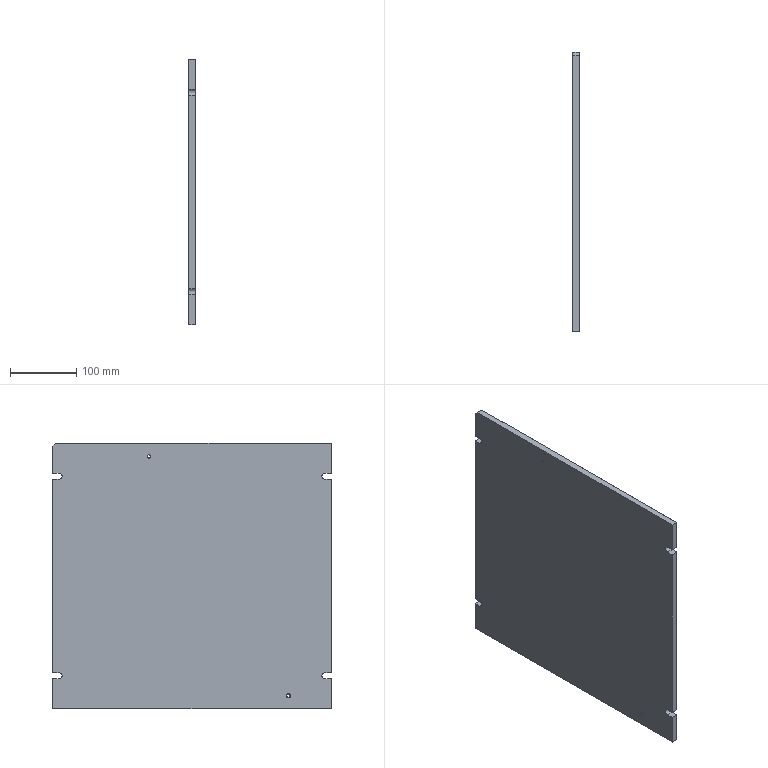Part | NX | 1 solid | 50 faces | box 10 x 420 x 400 mm | volume 1674456 mm3 | plane 38 | cylinder 8 | cone 4 | commonest cylinder face diameters 5 x4 9 x4
STEP:
#1=CARTESIAN_POINT('',(5.,-184.7,-204.5));
#2=VERTEX_POINT('',#1);
#3=CARTESIAN_POINT('',(5.,-184.7,-249.7));
#4=VERTEX_POINT('',#3);
#5=CARTESIAN_POINT('',(5.,-184.7,-227.25));
#6=DIRECTION('',(0.,0.,-1.));
#7=VECTOR('',#6,1000.);
#8=LINE('',#5,#7);
#9=EDGE_CURVE('',#2,#4,#8,.T.);
#10=ORIENTED_EDGE('',*,*,#9,.T.);
#11=CARTESIAN_POINT('',(5.,234.7,-249.7));
#12=VERTEX_POINT('',#11);
#13=CARTESIAN_POINT('',(5.,25.,-249.7));
#14=DIRECTION('',(0.,1.,0.));
#15=VECTOR('',#14,1000.);
#16=LINE('',#13,#15);
#17=EDGE_CURVE('',#4,#12,#16,.T.);
#18=ORIENTED_EDGE('',*,*,#17,.T.);
#19=CARTESIAN_POINT('',(5.,234.7,-204.5));
#20=VERTEX_POINT('',#19);
#21=CARTESIAN_POINT('',(5.,234.7,-227.25));
#22=DIRECTION('',(0.,0.,-1.));
#23=VECTOR('',#22,1000.);
#24=LINE('',#21,#23);
#25=EDGE_CURVE('',#20,#12,#24,.T.);
#26=ORIENTED_EDGE('',*,*,#25,.F.);
#27=CARTESIAN_POINT('',(5.,225.,-204.5));
#28=VERTEX_POINT('',#27);
#29=CARTESIAN_POINT('',(5.,0.,-204.5));
#30=DIRECTION('',(0.,1.,0.));
#31=VECTOR('',#30,1000.);
#32=LINE('',#29,#31);
#33=EDGE_CURVE('',#28,#20,#32,.T.);
#34=ORIENTED_EDGE('',*,*,#33,.F.);
#35=CARTESIAN_POINT('',(5.,225.,-195.5));
#36=VERTEX_POINT('',#35);
#37=CARTESIAN_POINT('',(5.,225.,-200.));
#38=DIRECTION('',(1.,0.,0.));
#39=DIRECTION('',(0.,0.,-1.));
#40=AXIS2_PLACEMENT_3D('',#37,#38,#39);
#41=CIRCLE('',#40,4.5);
#42=EDGE_CURVE('',#36,#28,#41,.T.);
#43=ORIENTED_EDGE('',*,*,#42,.F.);
#44=CARTESIAN_POINT('',(5.,234.7,-195.5));
#45=VERTEX_POINT('',#44);
#46=CARTESIAN_POINT('',(5.,0.,-195.5));
#47=DIRECTION('',(0.,-1.,0.));
#48=VECTOR('',#47,1000.);
#49=LINE('',#46,#48);
#50=EDGE_CURVE('',#45,#36,#49,.T.);
#51=ORIENTED_EDGE('',*,*,#50,.F.);
#52=CARTESIAN_POINT('',(5.,234.7,95.5));
#53=VERTEX_POINT('',#52);
#54=CARTESIAN_POINT('',(5.,234.7,-50.));
#55=DIRECTION('',(0.,0.,-1.));
#56=VECTOR('',#55,1000.);
#57=LINE('',#54,#56);
#58=EDGE_CURVE('',#53,#45,#57,.T.);
#59=ORIENTED_EDGE('',*,*,#58,.F.);
#60=CARTESIAN_POINT('',(5.,225.,95.5));
#61=VERTEX_POINT('',#60);
#62=CARTESIAN_POINT('',(5.,0.,95.5));
#63=DIRECTION('',(0.,1.,0.));
#64=VECTOR('',#63,1000.);
#65=LINE('',#62,#64);
#66=EDGE_CURVE('',#61,#53,#65,.T.);
#67=ORIENTED_EDGE('',*,*,#66,.F.);
#68=CARTESIAN_POINT('',(5.,225.,104.5));
#69=VERTEX_POINT('',#68);
#70=CARTESIAN_POINT('',(5.,225.,100.));
#71=DIRECTION('',(1.,0.,0.));
#72=DIRECTION('',(0.,0.,-1.));
#73=AXIS2_PLACEMENT_3D('',#70,#71,#72);
#74=CIRCLE('',#73,4.5);
#75=EDGE_CURVE('',#69,#61,#74,.T.);
#76=ORIENTED_EDGE('',*,*,#75,.F.);
#77=CARTESIAN_POINT('',(5.,234.7,104.5));
#78=VERTEX_POINT('',#77);
#79=CARTESIAN_POINT('',(5.,0.,104.5));
#80=DIRECTION('',(0.,-1.,0.));
#81=VECTOR('',#80,1000.);
#82=LINE('',#79,#81);
#83=EDGE_CURVE('',#78,#69,#82,.T.);
#84=ORIENTED_EDGE('',*,*,#83,.F.);
#85=CARTESIAN_POINT('',(5.,234.7,145.3));
#86=VERTEX_POINT('',#85);
#87=CARTESIAN_POINT('',(5.,234.7,124.75));
#88=DIRECTION('',(0.,0.,-1.));
#89=VECTOR('',#88,1000.);
#90=LINE('',#87,#89);
#91=EDGE_CURVE('',#86,#78,#90,.T.);
#92=ORIENTED_EDGE('',*,*,#91,.F.);
#93=CARTESIAN_POINT('',(5.,230.3,149.7));
#94=VERTEX_POINT('',#93);
#95=CARTESIAN_POINT('',(5.,380.,0.));
#96=DIRECTION('',(0.,0.7071,-0.7071));
#97=VECTOR('',#96,1000.);
#98=LINE('',#95,#97);
#99=EDGE_CURVE('',#94,#86,#98,.T.);
#100=ORIENTED_EDGE('',*,*,#99,.F.);
#101=CARTESIAN_POINT('',(5.,-184.7,149.7));
#102=VERTEX_POINT('',#101);
#103=CARTESIAN_POINT('',(5.,22.5,149.7));
#104=DIRECTION('',(0.,1.,0.));
#105=VECTOR('',#104,1000.);
#106=LINE('',#103,#105);
#107=EDGE_CURVE('',#102,#94,#106,.T.);
#108=ORIENTED_EDGE('',*,*,#107,.F.);
#109=CARTESIAN_POINT('',(5.,-184.7,104.5));
#110=VERTEX_POINT('',#109);
#111=CARTESIAN_POINT('',(5.,-184.7,127.25));
#112=DIRECTION('',(0.,0.,-1.));
#113=VECTOR('',#112,1000.);
#114=LINE('',#111,#113);
#115=EDGE_CURVE('',#102,#110,#114,.T.);
#116=ORIENTED_EDGE('',*,*,#115,.T.);
#117=CARTESIAN_POINT('',(5.,-175.,104.5));
#118=VERTEX_POINT('',#117);
#119=CARTESIAN_POINT('',(5.,0.,104.5));
#120=DIRECTION('',(0.,-1.,0.));
#121=VECTOR('',#120,1000.);
#122=LINE('',#119,#121);
#123=EDGE_CURVE('',#118,#110,#122,.T.);
#124=ORIENTED_EDGE('',*,*,#123,.F.);
#125=CARTESIAN_POINT('',(5.,-175.,95.5));
#126=VERTEX_POINT('',#125);
#127=CARTESIAN_POINT('',(5.,-175.,100.));
#128=DIRECTION('',(1.,0.,0.));
#129=DIRECTION('',(0.,0.,-1.));
#130=AXIS2_PLACEMENT_3D('',#127,#128,#129);
#131=CIRCLE('',#130,4.5);
#132=EDGE_CURVE('',#126,#118,#131,.T.);
#133=ORIENTED_EDGE('',*,*,#132,.F.);
#134=CARTESIAN_POINT('',(5.,-184.7,95.5));
#135=VERTEX_POINT('',#134);
#136=CARTESIAN_POINT('',(5.,0.,95.5));
#137=DIRECTION('',(0.,1.,0.));
#138=VECTOR('',#137,1000.);
#139=LINE('',#136,#138);
#140=EDGE_CURVE('',#135,#126,#139,.T.);
#141=ORIENTED_EDGE('',*,*,#140,.F.);
#142=CARTESIAN_POINT('',(5.,-184.7,-195.5));
#143=VERTEX_POINT('',#142);
#144=CARTESIAN_POINT('',(5.,-184.7,-50.));
#145=DIRECTION('',(0.,0.,-1.));
#146=VECTOR('',#145,1000.);
#147=LINE('',#144,#146);
#148=EDGE_CURVE('',#135,#143,#147,.T.);
#149=ORIENTED_EDGE('',*,*,#148,.T.);
#150=CARTESIAN_POINT('',(5.,-175.,-195.5));
#151=VERTEX_POINT('',#150);
#152=CARTESIAN_POINT('',(5.,0.,-195.5));
#153=DIRECTION('',(0.,-1.,0.));
#154=VECTOR('',#153,1000.);
#155=LINE('',#152,#154);
#156=EDGE_CURVE('',#151,#143,#155,.T.);
#157=ORIENTED_EDGE('',*,*,#156,.F.);
#158=CARTESIAN_POINT('',(5.,-175.,-204.5));
#159=VERTEX_POINT('',#158);
#160=CARTESIAN_POINT('',(5.,-175.,-200.));
#161=DIRECTION('',(1.,0.,0.));
#162=DIRECTION('',(0.,0.,-1.));
#163=AXIS2_PLACEMENT_3D('',#160,#161,#162);
#164=CIRCLE('',#163,4.5);
#165=EDGE_CURVE('',#159,#151,#164,.T.);
#166=ORIENTED_EDGE('',*,*,#165,.F.);
#167=CARTESIAN_POINT('',(5.,0.,-204.5));
#168=DIRECTION('',(0.,1.,0.));
#169=VECTOR('',#168,1000.);
#170=LINE('',#167,#169);
#171=EDGE_CURVE('',#2,#159,#170,.T.);
#172=ORIENTED_EDGE('',*,*,#171,.F.);
#173=EDGE_LOOP('',(#10,#18,#26,#34,#43,#51,#59,#67,#76,#84,#92,#100,#108,#116,#124,#133,#141,#149,#157,#166,#172));
#174=FACE_BOUND('',#173,.T.);
#175=CARTESIAN_POINT('',(5.,93.45,130.));
#176=VERTEX_POINT('',#175);
#177=CARTESIAN_POINT('',(5.,86.55,130.));
#178=VERTEX_POINT('',#177);
#179=CARTESIAN_POINT('',(5.,90.,130.));
#180=DIRECTION('',(1.,0.,0.));
#181=DIRECTION('',(0.,-1.,0.));
#182=AXIS2_PLACEMENT_3D('',#179,#180,#181);
#183=CIRCLE('',#182,3.45);
#184=EDGE_CURVE('',#176,#178,#183,.T.);
#185=ORIENTED_EDGE('',*,*,#184,.F.);
#186=CARTESIAN_POINT('',(5.,90.,130.));
#187=DIRECTION('',(1.,0.,0.));
#188=DIRECTION('',(0.,-1.,0.));
#189=AXIS2_PLACEMENT_3D('',#186,#187,#188);
#190=CIRCLE('',#189,3.45);
#191=EDGE_CURVE('',#178,#176,#190,.T.);
#192=ORIENTED_EDGE('',*,*,#191,.F.);
#193=EDGE_LOOP('',(#185,#192));
#194=FACE_BOUND('',#193,.T.);
#195=CARTESIAN_POINT('',(5.,-122.5,-230.));
#196=VERTEX_POINT('',#195);
#197=CARTESIAN_POINT('',(5.,-117.5,-230.));
#198=VERTEX_POINT('',#197);
#199=CARTESIAN_POINT('',(5.,-120.,-230.));
#200=DIRECTION('',(-1.,0.,0.));
#201=DIRECTION('',(0.,1.,0.));
#202=AXIS2_PLACEMENT_3D('',#199,#200,#201);
#203=CIRCLE('',#202,2.5);
#204=EDGE_CURVE('',#196,#198,#203,.T.);
#205=ORIENTED_EDGE('',*,*,#204,.T.);
#206=CARTESIAN_POINT('',(5.,-120.,-230.));
#207=DIRECTION('',(-1.,0.,0.));
#208=DIRECTION('',(0.,1.,0.));
#209=AXIS2_PLACEMENT_3D('',#206,#207,#208);
#210=CIRCLE('',#209,2.5);
#211=EDGE_CURVE('',#198,#196,#210,.T.);
#212=ORIENTED_EDGE('',*,*,#211,.T.);
#213=EDGE_LOOP('',(#205,#212));
#214=FACE_BOUND('',#213,.T.);
#215=CARTESIAN_POINT('',(5.,0.,0.));
#216=DIRECTION('',(1.,0.,0.));
#217=DIRECTION('',(0.,1.,0.));
#218=AXIS2_PLACEMENT_3D('',#215,#216,#217);
#219=PLANE('',#218);
#220=ADVANCED_FACE('',(#174,#194,#214),#219,.T.);
#221=CARTESIAN_POINT('',(-4.7,-184.7,150.));
#222=VERTEX_POINT('',#221);
#223=CARTESIAN_POINT('',(4.7,-184.7,150.));
#224=VERTEX_POINT('',#223);
#225=CARTESIAN_POINT('',(0.,-184.7,150.));
#226=DIRECTION('',(1.,0.,0.));
#227=VECTOR('',#226,1000.);
#228=LINE('',#225,#227);
#229=EDGE_CURVE('',#222,#224,#228,.T.);
#230=ORIENTED_EDGE('',*,*,#229,.T.);
#231=CARTESIAN_POINT('',(4.7,230.,150.));
#232=VERTEX_POINT('',#231);
#233=CARTESIAN_POINT('',(4.7,22.5,150.));
#234=DIRECTION('',(0.,1.,0.));
#235=VECTOR('',#234,1000.);
#236=LINE('',#233,#235);
#237=EDGE_CURVE('',#224,#232,#236,.T.);
#238=ORIENTED_EDGE('',*,*,#237,.T.);
#239=CARTESIAN_POINT('',(-4.7,230.,150.));
#240=VERTEX_POINT('',#239);
#241=CARTESIAN_POINT('',(5.,230.,150.));
#242=DIRECTION('',(-1.,0.,0.));
#243=VECTOR('',#242,1000.);
#244=LINE('',#241,#243);
#245=EDGE_CURVE('',#232,#240,#244,.T.);
#246=ORIENTED_EDGE('',*,*,#245,.T.);
#247=CARTESIAN_POINT('',(-4.7,22.5,150.));
#248=DIRECTION('',(0.,1.,0.));
#249=VECTOR('',#248,1000.);
#250=LINE('',#247,#249);
#251=EDGE_CURVE('',#222,#240,#250,.T.);
#252=ORIENTED_EDGE('',*,*,#251,.F.);
#253=EDGE_LOOP('',(#230,#238,#246,#252));
#254=FACE_BOUND('',#253,.T.);
#255=CARTESIAN_POINT('',(-5.,235.,150.));
#256=DIRECTION('',(0.,0.,1.));
#257=DIRECTION('',(1.,0.,0.));
#258=AXIS2_PLACEMENT_3D('',#255,#256,#257);
#259=PLANE('',#258);
#260=ADVANCED_FACE('',(#254),#259,.T.);
#261=ORIENTED_EDGE('',*,*,#245,.F.);
#262=CARTESIAN_POINT('',(154.7,380.,0.));
#263=DIRECTION('',(0.5774,0.5774,-0.5774));
#264=VECTOR('',#263,1000.);
#265=LINE('',#262,#264);
#266=EDGE_CURVE('',#232,#94,#265,.T.);
#267=ORIENTED_EDGE('',*,*,#266,.T.);
#268=ORIENTED_EDGE('',*,*,#99,.T.);
#269=CARTESIAN_POINT('',(4.7,235.,145.));
#270=VERTEX_POINT('',#269);
#271=CARTESIAN_POINT('',(239.7,0.,380.));
#272=DIRECTION('',(-0.5774,0.5774,-0.5774));
#273=VECTOR('',#272,1000.);
#274=LINE('',#271,#273);
#275=EDGE_CURVE('',#86,#270,#274,.T.);
#276=ORIENTED_EDGE('',*,*,#275,.T.);
#277=CARTESIAN_POINT('',(-4.7,235.,145.));
#278=VERTEX_POINT('',#277);
#279=CARTESIAN_POINT('',(5.,235.,145.));
#280=DIRECTION('',(-1.,0.,0.));
#281=VECTOR('',#280,1000.);
#282=LINE('',#279,#281);
#283=EDGE_CURVE('',#270,#278,#282,.T.);
#284=ORIENTED_EDGE('',*,*,#283,.T.);
#285=CARTESIAN_POINT('',(-5.,234.7,145.3));
#286=VERTEX_POINT('',#285);
#287=CARTESIAN_POINT('',(140.3,380.,0.));
#288=DIRECTION('',(0.5774,0.5774,-0.5774));
#289=VECTOR('',#288,1000.);
#290=LINE('',#287,#289);
#291=EDGE_CURVE('',#286,#278,#290,.T.);
#292=ORIENTED_EDGE('',*,*,#291,.F.);
#293=CARTESIAN_POINT('',(-5.,230.3,149.7));
#294=VERTEX_POINT('',#293);
#295=CARTESIAN_POINT('',(-5.,380.,0.));
#296=DIRECTION('',(0.,0.7071,-0.7071));
#297=VECTOR('',#296,1000.);
#298=LINE('',#295,#297);
#299=EDGE_CURVE('',#294,#286,#298,.T.);
#300=ORIENTED_EDGE('',*,*,#299,.F.);
#301=CARTESIAN_POINT('',(-154.7,380.,0.));
#302=DIRECTION('',(-0.5774,0.5774,-0.5774));
#303=VECTOR('',#302,1000.);
#304=LINE('',#301,#303);
#305=EDGE_CURVE('',#240,#294,#304,.T.);
#306=ORIENTED_EDGE('',*,*,#305,.F.);
#307=EDGE_LOOP('',(#261,#267,#268,#276,#284,#292,#300,#306));
#308=FACE_BOUND('',#307,.T.);
#309=CARTESIAN_POINT('',(-5.,230.,150.));
#310=DIRECTION('',(0.,0.7071,0.7071));
#311=DIRECTION('',(1.,0.,0.));
#312=AXIS2_PLACEMENT_3D('',#309,#310,#311);
#313=PLANE('',#312);
#314=ADVANCED_FACE('',(#308),#313,.T.);
#315=CARTESIAN_POINT('',(4.7,235.,-249.7));
#316=VERTEX_POINT('',#315);
#317=CARTESIAN_POINT('',(-4.7,235.,-249.7));
#318=VERTEX_POINT('',#317);
#319=CARTESIAN_POINT('',(0.,235.,-249.7));
#320=DIRECTION('',(-1.,0.,0.));
#321=VECTOR('',#320,1000.);
#322=LINE('',#319,#321);
#323=EDGE_CURVE('',#316,#318,#322,.T.);
#324=ORIENTED_EDGE('',*,*,#323,.T.);
#325=CARTESIAN_POINT('',(-4.7,235.,-204.5));
#326=VERTEX_POINT('',#325);
#327=CARTESIAN_POINT('',(-4.7,235.,-227.25));
#328=DIRECTION('',(0.,0.,-1.));
#329=VECTOR('',#328,1000.);
#330=LINE('',#327,#329);
#331=EDGE_CURVE('',#326,#318,#330,.T.);
#332=ORIENTED_EDGE('',*,*,#331,.F.);
#333=CARTESIAN_POINT('',(4.7,235.,-204.5));
#334=VERTEX_POINT('',#333);
#335=CARTESIAN_POINT('',(-6.,235.,-204.5));
#336=DIRECTION('',(1.,0.,0.));
#337=VECTOR('',#336,1000.);
#338=LINE('',#335,#337);
#339=EDGE_CURVE('',#326,#334,#338,.T.);
#340=ORIENTED_EDGE('',*,*,#339,.T.);
#341=CARTESIAN_POINT('',(4.7,235.,-227.25));
#342=DIRECTION('',(0.,0.,-1.));
#343=VECTOR('',#342,1000.);
#344=LINE('',#341,#343);
#345=EDGE_CURVE('',#334,#316,#344,.T.);
#346=ORIENTED_EDGE('',*,*,#345,.T.);
#347=EDGE_LOOP('',(#324,#332,#340,#346));
#348=FACE_BOUND('',#347,.T.);
#349=CARTESIAN_POINT('',(-5.,235.,-150.));
#350=DIRECTION('',(0.,1.,0.));
#351=DIRECTION('',(1.,0.,0.));
#352=AXIS2_PLACEMENT_3D('',#349,#350,#351);
#353=PLANE('',#352);
#354=ADVANCED_FACE('',(#348),#353,.T.);
#355=CARTESIAN_POINT('',(-4.7,235.,104.5));
#356=VERTEX_POINT('',#355);
#357=CARTESIAN_POINT('',(4.7,235.,104.5));
#358=VERTEX_POINT('',#357);
#359=CARTESIAN_POINT('',(-6.,235.,104.5));
#360=DIRECTION('',(1.,0.,0.));
#361=VECTOR('',#360,1000.);
#362=LINE('',#359,#361);
#363=EDGE_CURVE('',#356,#358,#362,.T.);
#364=ORIENTED_EDGE('',*,*,#363,.F.);
#365=CARTESIAN_POINT('',(-4.7,235.,124.75));
#366=DIRECTION('',(0.,0.,-1.));
#367=VECTOR('',#366,1000.);
#368=LINE('',#365,#367);
#369=EDGE_CURVE('',#278,#356,#368,.T.);
#370=ORIENTED_EDGE('',*,*,#369,.F.);
#371=ORIENTED_EDGE('',*,*,#283,.F.);
#372=CARTESIAN_POINT('',(4.7,235.,124.75));
#373=DIRECTION('',(0.,0.,-1.));
#374=VECTOR('',#373,1000.);
#375=LINE('',#372,#374);
#376=EDGE_CURVE('',#270,#358,#375,.T.);
#377=ORIENTED_EDGE('',*,*,#376,.T.);
#378=EDGE_LOOP('',(#364,#370,#371,#377));
#379=FACE_BOUND('',#378,.T.);
#380=CARTESIAN_POINT('',(-5.,235.,-150.));
#381=DIRECTION('',(0.,1.,0.));
#382=DIRECTION('',(1.,0.,0.));
#383=AXIS2_PLACEMENT_3D('',#380,#381,#382);
#384=PLANE('',#383);
#385=ADVANCED_FACE('',(#379),#384,.T.);
#386=CARTESIAN_POINT('',(4.7,-184.7,-250.));
#387=VERTEX_POINT('',#386);
#388=CARTESIAN_POINT('',(-4.7,-184.7,-250.));
#389=VERTEX_POINT('',#388);
#390=CARTESIAN_POINT('',(0.,-184.7,-250.));
#391=DIRECTION('',(-1.,0.,0.));
#392=VECTOR('',#391,1000.);
#393=LINE('',#390,#392);
#394=EDGE_CURVE('',#387,#389,#393,.T.);
#395=ORIENTED_EDGE('',*,*,#394,.T.);
#396=CARTESIAN_POINT('',(-4.7,234.7,-250.));
#397=VERTEX_POINT('',#396);
#398=CARTESIAN_POINT('',(-4.7,25.,-250.));
#399=DIRECTION('',(0.,1.,0.));
#400=VECTOR('',#399,1000.);
#401=LINE('',#398,#400);
#402=EDGE_CURVE('',#389,#397,#401,.T.);
#403=ORIENTED_EDGE('',*,*,#402,.T.);
#404=CARTESIAN_POINT('',(4.7,234.7,-250.));
#405=VERTEX_POINT('',#404);
#406=CARTESIAN_POINT('',(0.,234.7,-250.));
#407=DIRECTION('',(-1.,0.,0.));
#408=VECTOR('',#407,1000.);
#409=LINE('',#406,#408);
#410=EDGE_CURVE('',#405,#397,#409,.T.);
#411=ORIENTED_EDGE('',*,*,#410,.F.);
#412=CARTESIAN_POINT('',(4.7,25.,-250.));
#413=DIRECTION('',(0.,1.,0.));
#414=VECTOR('',#413,1000.);
#415=LINE('',#412,#414);
#416=EDGE_CURVE('',#387,#405,#415,.T.);
#417=ORIENTED_EDGE('',*,*,#416,.F.);
#418=EDGE_LOOP('',(#395,#403,#411,#417));
#419=FACE_BOUND('',#418,.T.);
#420=CARTESIAN_POINT('',(-5.,-235.,-250.));
#421=DIRECTION('',(0.,0.,-1.));
#422=DIRECTION('',(0.,-1.,0.));
#423=AXIS2_PLACEMENT_3D('',#420,#421,#422);
#424=PLANE('',#423);
#425=ADVANCED_FACE('',(#419),#424,.T.);
#426=CARTESIAN_POINT('',(-5.,225.,-204.5));
#427=VERTEX_POINT('',#426);
#428=CARTESIAN_POINT('',(-5.,234.7,-204.5));
#429=VERTEX_POINT('',#428);
#430=CARTESIAN_POINT('',(-5.,0.,-204.5));
#431=DIRECTION('',(0.,1.,0.));
#432=VECTOR('',#431,1000.);
#433=LINE('',#430,#432);
#434=EDGE_CURVE('',#427,#429,#433,.T.);
#435=ORIENTED_EDGE('',*,*,#434,.F.);
#436=CARTESIAN_POINT('',(-6.,225.,-204.5));
#437=DIRECTION('',(1.,0.,0.));
#438=VECTOR('',#437,1000.);
#439=LINE('',#436,#438);
#440=EDGE_CURVE('',#427,#28,#439,.T.);
#441=ORIENTED_EDGE('',*,*,#440,.T.);
#442=ORIENTED_EDGE('',*,*,#33,.T.);
#443=CARTESIAN_POINT('',(239.7,0.,-204.5));
#444=DIRECTION('',(0.7071,-0.7071,0.));
#445=VECTOR('',#444,1000.);
#446=LINE('',#443,#445);
#447=EDGE_CURVE('',#334,#20,#446,.T.);
#448=ORIENTED_EDGE('',*,*,#447,.F.);
#449=ORIENTED_EDGE('',*,*,#339,.F.);
#450=CARTESIAN_POINT('',(-239.7,0.,-204.5));
#451=DIRECTION('',(-0.7071,-0.7071,0.));
#452=VECTOR('',#451,1000.);
#453=LINE('',#450,#452);
#454=EDGE_CURVE('',#326,#429,#453,.T.);
#455=ORIENTED_EDGE('',*,*,#454,.T.);
#456=EDGE_LOOP('',(#435,#441,#442,#448,#449,#455));
#457=FACE_BOUND('',#456,.T.);
#458=CARTESIAN_POINT('',(-6.,235.,-204.5));
#459=DIRECTION('',(0.,0.,-1.));
#460=DIRECTION('',(0.,-1.,0.));
#461=AXIS2_PLACEMENT_3D('',#458,#459,#460);
#462=PLANE('',#461);
#463=ADVANCED_FACE('',(#457),#462,.F.);
#464=CARTESIAN_POINT('',(-4.7,-185.,-204.5));
#465=VERTEX_POINT('',#464);
#466=CARTESIAN_POINT('',(-4.7,-185.,-249.7));
#467=VERTEX_POINT('',#466);
#468=CARTESIAN_POINT('',(-4.7,-185.,-227.25));
#469=DIRECTION('',(0.,0.,-1.));
#470=VECTOR('',#469,1000.);
#471=LINE('',#468,#470);
#472=EDGE_CURVE('',#465,#467,#471,.T.);
#473=ORIENTED_EDGE('',*,*,#472,.T.);
#474=CARTESIAN_POINT('',(4.7,-185.,-249.7));
#475=VERTEX_POINT('',#474);
#476=CARTESIAN_POINT('',(0.,-185.,-249.7));
#477=DIRECTION('',(-1.,0.,0.));
#478=VECTOR('',#477,1000.);
#479=LINE('',#476,#478);
#480=EDGE_CURVE('',#475,#467,#479,.T.);
#481=ORIENTED_EDGE('',*,*,#480,.F.);
#482=CARTESIAN_POINT('',(4.7,-185.,-204.5));
#483=VERTEX_POINT('',#482);
#484=CARTESIAN_POINT('',(4.7,-185.,-227.25));
#485=DIRECTION('',(0.,0.,-1.));
#486=VECTOR('',#485,1000.);
#487=LINE('',#484,#486);
#488=EDGE_CURVE('',#483,#475,#487,.T.);
#489=ORIENTED_EDGE('',*,*,#488,.F.);
#490=CARTESIAN_POINT('',(0.,-185.,-204.5));
#491=DIRECTION('',(-1.,0.,0.));
#492=VECTOR('',#491,1000.);
#493=LINE('',#490,#492);
#494=EDGE_CURVE('',#483,#465,#493,.T.);
#495=ORIENTED_EDGE('',*,*,#494,.T.);
#496=EDGE_LOOP('',(#473,#481,#489,#495));
#497=FACE_BOUND('',#496,.T.);
#498=CARTESIAN_POINT('',(-5.,-185.,150.));
#499=DIRECTION('',(0.,-1.,0.));
#500=DIRECTION('',(0.,0.,-1.));
#501=AXIS2_PLACEMENT_3D('',#498,#499,#500);
#502=PLANE('',#501);
#503=ADVANCED_FACE('',(#497),#502,.T.);
#504=CARTESIAN_POINT('',(4.452,92.5,130.));
#505=VERTEX_POINT('',#504);
#506=CARTESIAN_POINT('',(4.452,87.5,130.));
#507=VERTEX_POINT('',#506);
#508=CARTESIAN_POINT('',(4.452,90.,130.));
#509=DIRECTION('',(1.,0.,0.));
#510=DIRECTION('',(0.,-1.,0.));
#511=AXIS2_PLACEMENT_3D('',#508,#509,#510);
#512=CIRCLE('',#511,2.5);
#513=EDGE_CURVE('',#505,#507,#512,.T.);
#514=ORIENTED_EDGE('',*,*,#513,.T.);
#515=CARTESIAN_POINT('',(-5.,87.5,130.));
#516=VERTEX_POINT('',#515);
#517=CARTESIAN_POINT('',(5.,87.5,130.));
#518=DIRECTION('',(1.,0.,0.));
#519=VECTOR('',#518,1000.);
#520=LINE('',#517,#519);
#521=EDGE_CURVE('',#507,#516,#520,.F.);
#522=ORIENTED_EDGE('',*,*,#521,.T.);
#523=CARTESIAN_POINT('',(-5.,92.5,130.));
#524=VERTEX_POINT('',#523);
#525=CARTESIAN_POINT('',(-5.,90.,130.));
#526=DIRECTION('',(1.,0.,0.));
#527=DIRECTION('',(0.,-1.,0.));
#528=AXIS2_PLACEMENT_3D('',#525,#526,#527);
#529=CIRCLE('',#528,2.5);
#530=EDGE_CURVE('',#524,#516,#529,.T.);
#531=ORIENTED_EDGE('',*,*,#530,.F.);
#532=CARTESIAN_POINT('',(5.,92.5,130.));
#533=DIRECTION('',(1.,0.,0.));
#534=VECTOR('',#533,1000.);
#535=LINE('',#532,#534);
#536=EDGE_CURVE('',#505,#524,#535,.F.);
#537=ORIENTED_EDGE('',*,*,#536,.F.);
#538=EDGE_LOOP('',(#514,#522,#531,#537));
#539=FACE_BOUND('',#538,.T.);
#540=CARTESIAN_POINT('',(5.,90.,130.));
#541=DIRECTION('',(1.,0.,0.));
#542=DIRECTION('',(0.,-1.,0.));
#543=AXIS2_PLACEMENT_3D('',#540,#541,#542);
#544=CYLINDRICAL_SURFACE('',#543,2.5);
#545=ADVANCED_FACE('',(#539),#544,.F.);
#546=CARTESIAN_POINT('',(-5.,-184.7,-204.5));
#547=VERTEX_POINT('',#546);
#548=CARTESIAN_POINT('',(-5.,-184.7,-249.7));
#549=VERTEX_POINT('',#548);
#550=CARTESIAN_POINT('',(-5.,-184.7,-227.25));
#551=DIRECTION('',(0.,0.,-1.));
#552=VECTOR('',#551,1000.);
#553=LINE('',#550,#552);
#554=EDGE_CURVE('',#547,#549,#553,.T.);
#555=ORIENTED_EDGE('',*,*,#554,.F.);
#556=CARTESIAN_POINT('',(-5.,-175.,-204.5));
#557=VERTEX_POINT('',#556);
#558=CARTESIAN_POINT('',(-5.,0.,-204.5));
#559=DIRECTION('',(0.,1.,0.));
#560=VECTOR('',#559,1000.);
#561=LINE('',#558,#560);
#562=EDGE_CURVE('',#547,#557,#561,.T.);
#563=ORIENTED_EDGE('',*,*,#562,.T.);
#564=CARTESIAN_POINT('',(-5.,-175.,-195.5));
#565=VERTEX_POINT('',#564);
#566=CARTESIAN_POINT('',(-5.,-175.,-200.));
#567=DIRECTION('',(1.,0.,0.));
#568=DIRECTION('',(0.,0.,-1.));
#569=AXIS2_PLACEMENT_3D('',#566,#567,#568);
#570=CIRCLE('',#569,4.5);
#571=EDGE_CURVE('',#557,#565,#570,.T.);
#572=ORIENTED_EDGE('',*,*,#571,.T.);
#573=CARTESIAN_POINT('',(-5.,-184.7,-195.5));
#574=VERTEX_POINT('',#573);
#575=CARTESIAN_POINT('',(-5.,0.,-195.5));
#576=DIRECTION('',(0.,-1.,0.));
#577=VECTOR('',#576,1000.);
#578=LINE('',#575,#577);
#579=EDGE_CURVE('',#565,#574,#578,.T.);
#580=ORIENTED_EDGE('',*,*,#579,.T.);
#581=CARTESIAN_POINT('',(-5.,-184.7,95.5));
#582=VERTEX_POINT('',#581);
#583=CARTESIAN_POINT('',(-5.,-184.7,-50.));
#584=DIRECTION('',(0.,0.,-1.));
#585=VECTOR('',#584,1000.);
#586=LINE('',#583,#585);
#587=EDGE_CURVE('',#582,#574,#586,.T.);
#588=ORIENTED_EDGE('',*,*,#587,.F.);
#589=CARTESIAN_POINT('',(-5.,-175.,95.5));
#590=VERTEX_POINT('',#589);
#591=CARTESIAN_POINT('',(-5.,0.,95.5));
#592=DIRECTION('',(0.,1.,0.));
#593=VECTOR('',#592,1000.);
#594=LINE('',#591,#593);
#595=EDGE_CURVE('',#582,#590,#594,.T.);
#596=ORIENTED_EDGE('',*,*,#595,.T.);
#597=CARTESIAN_POINT('',(-5.,-175.,104.5));
#598=VERTEX_POINT('',#597);
#599=CARTESIAN_POINT('',(-5.,-175.,100.));
#600=DIRECTION('',(1.,0.,0.));
#601=DIRECTION('',(0.,0.,-1.));
#602=AXIS2_PLACEMENT_3D('',#599,#600,#601);
#603=CIRCLE('',#602,4.5);
#604=EDGE_CURVE('',#590,#598,#603,.T.);
#605=ORIENTED_EDGE('',*,*,#604,.T.);
#606=CARTESIAN_POINT('',(-5.,-184.7,104.5));
#607=VERTEX_POINT('',#606);
#608=CARTESIAN_POINT('',(-5.,0.,104.5));
#609=DIRECTION('',(0.,-1.,0.));
#610=VECTOR('',#609,1000.);
#611=LINE('',#608,#610);
#612=EDGE_CURVE('',#598,#607,#611,.T.);
#613=ORIENTED_EDGE('',*,*,#612,.T.);
#614=CARTESIAN_POINT('',(-5.,-184.7,149.7));
#615=VERTEX_POINT('',#614);
#616=CARTESIAN_POINT('',(-5.,-184.7,127.25));
#617=DIRECTION('',(0.,0.,-1.));
#618=VECTOR('',#617,1000.);
#619=LINE('',#616,#618);
#620=EDGE_CURVE('',#615,#607,#619,.T.);
#621=ORIENTED_EDGE('',*,*,#620,.F.);
#622=CARTESIAN_POINT('',(-5.,22.5,149.7));
#623=DIRECTION('',(0.,1.,0.));
#624=VECTOR('',#623,1000.);
#625=LINE('',#622,#624);
#626=EDGE_CURVE('',#615,#294,#625,.T.);
#627=ORIENTED_EDGE('',*,*,#626,.T.);
#628=ORIENTED_EDGE('',*,*,#299,.T.);
#629=CARTESIAN_POINT('',(-5.,234.7,104.5));
#630=VERTEX_POINT('',#629);
#631=CARTESIAN_POINT('',(-5.,234.7,124.75));
#632=DIRECTION('',(0.,0.,-1.));
#633=VECTOR('',#632,1000.);
#634=LINE('',#631,#633);
#635=EDGE_CURVE('',#286,#630,#634,.T.);
#636=ORIENTED_EDGE('',*,*,#635,.T.);
#637=CARTESIAN_POINT('',(-5.,225.,104.5));
#638=VERTEX_POINT('',#637);
#639=CARTESIAN_POINT('',(-5.,0.,104.5));
#640=DIRECTION('',(0.,-1.,0.));
#641=VECTOR('',#640,1000.);
#642=LINE('',#639,#641);
#643=EDGE_CURVE('',#630,#638,#642,.T.);
#644=ORIENTED_EDGE('',*,*,#643,.T.);
#645=CARTESIAN_POINT('',(-5.,225.,95.5));
#646=VERTEX_POINT('',#645);
#647=CARTESIAN_POINT('',(-5.,225.,100.));
#648=DIRECTION('',(1.,0.,0.));
#649=DIRECTION('',(0.,0.,-1.));
#650=AXIS2_PLACEMENT_3D('',#647,#648,#649);
#651=CIRCLE('',#650,4.5);
#652=EDGE_CURVE('',#638,#646,#651,.T.);
#653=ORIENTED_EDGE('',*,*,#652,.T.);
#654=CARTESIAN_POINT('',(-5.,234.7,95.5));
#655=VERTEX_POINT('',#654);
#656=CARTESIAN_POINT('',(-5.,0.,95.5));
#657=DIRECTION('',(0.,1.,0.));
#658=VECTOR('',#657,1000.);
#659=LINE('',#656,#658);
#660=EDGE_CURVE('',#646,#655,#659,.T.);
#661=ORIENTED_EDGE('',*,*,#660,.T.);
#662=CARTESIAN_POINT('',(-5.,234.7,-195.5));
#663=VERTEX_POINT('',#662);
#664=CARTESIAN_POINT('',(-5.,234.7,-50.));
#665=DIRECTION('',(0.,0.,-1.));
#666=VECTOR('',#665,1000.);
#667=LINE('',#664,#666);
#668=EDGE_CURVE('',#655,#663,#667,.T.);
#669=ORIENTED_EDGE('',*,*,#668,.T.);
#670=CARTESIAN_POINT('',(-5.,225.,-195.5));
#671=VERTEX_POINT('',#670);
#672=CARTESIAN_POINT('',(-5.,0.,-195.5));
#673=DIRECTION('',(0.,-1.,0.));
#674=VECTOR('',#673,1000.);
#675=LINE('',#672,#674);
#676=EDGE_CURVE('',#663,#671,#675,.T.);
#677=ORIENTED_EDGE('',*,*,#676,.T.);
#678=CARTESIAN_POINT('',(-5.,225.,-200.));
#679=DIRECTION('',(1.,0.,0.));
#680=DIRECTION('',(0.,0.,-1.));
#681=AXIS2_PLACEMENT_3D('',#678,#679,#680);
#682=CIRCLE('',#681,4.5);
#683=EDGE_CURVE('',#671,#427,#682,.T.);
#684=ORIENTED_EDGE('',*,*,#683,.T.);
#685=ORIENTED_EDGE('',*,*,#434,.T.);
#686=CARTESIAN_POINT('',(-5.,234.7,-249.7));
#687=VERTEX_POINT('',#686);
#688=CARTESIAN_POINT('',(-5.,234.7,-227.25));
#689=DIRECTION('',(0.,0.,-1.));
#690=VECTOR('',#689,1000.);
#691=LINE('',#688,#690);
#692=EDGE_CURVE('',#429,#687,#691,.T.);
#693=ORIENTED_EDGE('',*,*,#692,.T.);
#694=CARTESIAN_POINT('',(-5.,25.,-249.7));
#695=DIRECTION('',(0.,1.,0.));
#696=VECTOR('',#695,1000.);
#697=LINE('',#694,#696);
#698=EDGE_CURVE('',#549,#687,#697,.T.);
#699=ORIENTED_EDGE('',*,*,#698,.F.);
#700=EDGE_LOOP('',(#555,#563,#572,#580,#588,#596,#605,#613,#621,#627,#628,#636,#644,#653,#661,#669,#677,#684,#685,#693,#699));
#701=FACE_BOUND('',#700,.T.);
#702=CARTESIAN_POINT('',(-5.,-123.45,-230.));
#703=VERTEX_POINT('',#702);
#704=CARTESIAN_POINT('',(-5.,-116.55,-230.));
#705=VERTEX_POINT('',#704);
#706=CARTESIAN_POINT('',(-5.,-120.,-230.));
#707=DIRECTION('',(-1.,0.,0.));
#708=DIRECTION('',(0.,1.,0.));
#709=AXIS2_PLACEMENT_3D('',#706,#707,#708);
#710=CIRCLE('',#709,3.45);
#711=EDGE_CURVE('',#703,#705,#710,.T.);
#712=ORIENTED_EDGE('',*,*,#711,.F.);
#713=CARTESIAN_POINT('',(-5.,-120.,-230.));
#714=DIRECTION('',(-1.,0.,0.));
#715=DIRECTION('',(0.,1.,0.));
#716=AXIS2_PLACEMENT_3D('',#713,#714,#715);
#717=CIRCLE('',#716,3.45);
#718=EDGE_CURVE('',#705,#703,#717,.T.);
#719=ORIENTED_EDGE('',*,*,#718,.F.);
#720=EDGE_LOOP('',(#712,#719));
#721=FACE_BOUND('',#720,.T.);
#722=ORIENTED_EDGE('',*,*,#530,.T.);
#723=CARTESIAN_POINT('',(-5.,90.,130.));
#724=DIRECTION('',(1.,0.,0.));
#725=DIRECTION('',(0.,-1.,0.));
#726=AXIS2_PLACEMENT_3D('',#723,#724,#725);
#727=CIRCLE('',#726,2.5);
#728=EDGE_CURVE('',#516,#524,#727,.T.);
#729=ORIENTED_EDGE('',*,*,#728,.T.);
#730=EDGE_LOOP('',(#722,#729));
#731=FACE_BOUND('',#730,.T.);
#732=CARTESIAN_POINT('',(-5.,0.,0.));
#733=DIRECTION('',(1.,0.,0.));
#734=DIRECTION('',(0.,1.,0.));
#735=AXIS2_PLACEMENT_3D('',#732,#733,#734);
#736=PLANE('',#735);
#737=ADVANCED_FACE('',(#701,#721,#731),#736,.F.);
#738=CARTESIAN_POINT('',(-4.7,-185.,-195.5));
#739=VERTEX_POINT('',#738);
#740=CARTESIAN_POINT('',(4.7,-185.,-195.5));
#741=VERTEX_POINT('',#740);
#742=CARTESIAN_POINT('',(0.,-185.,-195.5));
#743=DIRECTION('',(1.,0.,0.));
#744=VECTOR('',#743,1000.);
#745=LINE('',#742,#744);
#746=EDGE_CURVE('',#739,#741,#745,.T.);
#747=ORIENTED_EDGE('',*,*,#746,.T.);
#748=CARTESIAN_POINT('',(4.7,-185.,95.5));
#749=VERTEX_POINT('',#748);
#750=CARTESIAN_POINT('',(4.7,-185.,-50.));
#751=DIRECTION('',(0.,0.,-1.));
#752=VECTOR('',#751,1000.);
#753=LINE('',#750,#752);
#754=EDGE_CURVE('',#749,#741,#753,.T.);
#755=ORIENTED_EDGE('',*,*,#754,.F.);
#756=CARTESIAN_POINT('',(-4.7,-185.,95.5));
#757=VERTEX_POINT('',#756);
#758=CARTESIAN_POINT('',(0.,-185.,95.5));
#759=DIRECTION('',(-1.,0.,0.));
#760=VECTOR('',#759,1000.);
#761=LINE('',#758,#760);
#762=EDGE_CURVE('',#749,#757,#761,.T.);
#763=ORIENTED_EDGE('',*,*,#762,.T.);
#764=CARTESIAN_POINT('',(-4.7,-185.,-50.));
#765=DIRECTION('',(0.,0.,-1.));
#766=VECTOR('',#765,1000.);
#767=LINE('',#764,#766);
#768=EDGE_CURVE('',#757,#739,#767,.T.);
#769=ORIENTED_EDGE('',*,*,#768,.T.);
#770=EDGE_LOOP('',(#747,#755,#763,#769));
#771=FACE_BOUND('',#770,.T.);
#772=CARTESIAN_POINT('',(-5.,-185.,150.));
#773=DIRECTION('',(0.,-1.,0.));
#774=DIRECTION('',(0.,0.,-1.));
#775=AXIS2_PLACEMENT_3D('',#772,#773,#774);
#776=PLANE('',#775);
#777=ADVANCED_FACE('',(#771),#776,.T.);
#778=CARTESIAN_POINT('',(-4.7,-185.,149.7));
#779=VERTEX_POINT('',#778);
#780=CARTESIAN_POINT('',(4.7,-185.,149.7));
#781=VERTEX_POINT('',#780);
#782=CARTESIAN_POINT('',(0.,-185.,149.7));
#783=DIRECTION('',(1.,0.,0.));
#784=VECTOR('',#783,1000.);
#785=LINE('',#782,#784);
#786=EDGE_CURVE('',#779,#781,#785,.T.);
#787=ORIENTED_EDGE('',*,*,#786,.F.);
#788=CARTESIAN_POINT('',(-4.7,-185.,104.5));
#789=VERTEX_POINT('',#788);
#790=CARTESIAN_POINT('',(-4.7,-185.,127.25));
#791=DIRECTION('',(0.,0.,-1.));
#792=VECTOR('',#791,1000.);
#793=LINE('',#790,#792);
#794=EDGE_CURVE('',#779,#789,#793,.T.);
#795=ORIENTED_EDGE('',*,*,#794,.T.);
#796=CARTESIAN_POINT('',(4.7,-185.,104.5));
#797=VERTEX_POINT('',#796);
#798=CARTESIAN_POINT('',(0.,-185.,104.5));
#799=DIRECTION('',(1.,0.,0.));
#800=VECTOR('',#799,1000.);
#801=LINE('',#798,#800);
#802=EDGE_CURVE('',#789,#797,#801,.T.);
#803=ORIENTED_EDGE('',*,*,#802,.T.);
#804=CARTESIAN_POINT('',(4.7,-185.,127.25));
#805=DIRECTION('',(0.,0.,-1.));
#806=VECTOR('',#805,1000.);
#807=LINE('',#804,#806);
#808=EDGE_CURVE('',#781,#797,#807,.T.);
#809=ORIENTED_EDGE('',*,*,#808,.F.);
#810=EDGE_LOOP('',(#787,#795,#803,#809));
#811=FACE_BOUND('',#810,.T.);
#812=CARTESIAN_POINT('',(-5.,-185.,150.));
#813=DIRECTION('',(0.,-1.,0.));
#814=DIRECTION('',(0.,0.,-1.));
#815=AXIS2_PLACEMENT_3D('',#812,#813,#814);
#816=PLANE('',#815);
#817=ADVANCED_FACE('',(#811),#816,.T.);
#818=CARTESIAN_POINT('',(4.7,235.,95.5));
#819=VERTEX_POINT('',#818);
#820=CARTESIAN_POINT('',(-4.7,235.,95.5));
#821=VERTEX_POINT('',#820);
#822=CARTESIAN_POINT('',(0.,235.,95.5));
#823=DIRECTION('',(-1.,0.,0.));
#824=VECTOR('',#823,1000.);
#825=LINE('',#822,#824);
#826=EDGE_CURVE('',#819,#821,#825,.T.);
#827=ORIENTED_EDGE('',*,*,#826,.F.);
#828=CARTESIAN_POINT('',(4.7,235.,-195.5));
#829=VERTEX_POINT('',#828);
#830=CARTESIAN_POINT('',(4.7,235.,-50.));
#831=DIRECTION('',(0.,0.,-1.));
#832=VECTOR('',#831,1000.);
#833=LINE('',#830,#832);
#834=EDGE_CURVE('',#819,#829,#833,.T.);
#835=ORIENTED_EDGE('',*,*,#834,.T.);
#836=CARTESIAN_POINT('',(-4.7,235.,-195.5));
#837=VERTEX_POINT('',#836);
#838=CARTESIAN_POINT('',(-6.,235.,-195.5));
#839=DIRECTION('',(1.,0.,0.));
#840=VECTOR('',#839,1000.);
#841=LINE('',#838,#840);
#842=EDGE_CURVE('',#837,#829,#841,.T.);
#843=ORIENTED_EDGE('',*,*,#842,.F.);
#844=CARTESIAN_POINT('',(-4.7,235.,-50.));
#845=DIRECTION('',(0.,0.,-1.));
#846=VECTOR('',#845,1000.);
#847=LINE('',#844,#846);
#848=EDGE_CURVE('',#821,#837,#847,.T.);
#849=ORIENTED_EDGE('',*,*,#848,.F.);
#850=EDGE_LOOP('',(#827,#835,#843,#849));
#851=FACE_BOUND('',#850,.T.);
#852=CARTESIAN_POINT('',(-5.,235.,-150.));
#853=DIRECTION('',(0.,1.,0.));
#854=DIRECTION('',(1.,0.,0.));
#855=AXIS2_PLACEMENT_3D('',#852,#853,#854);
#856=PLANE('',#855);
#857=ADVANCED_FACE('',(#851),#856,.T.);
#858=ORIENTED_EDGE('',*,*,#643,.F.);
#859=CARTESIAN_POINT('',(-239.7,0.,104.5));
#860=DIRECTION('',(0.7071,0.7071,0.));
#861=VECTOR('',#860,1000.);
#862=LINE('',#859,#861);
#863=EDGE_CURVE('',#630,#356,#862,.T.);
#864=ORIENTED_EDGE('',*,*,#863,.T.);
#865=ORIENTED_EDGE('',*,*,#363,.T.);
#866=CARTESIAN_POINT('',(239.7,0.,104.5));
#867=DIRECTION('',(-0.7071,0.7071,0.));
#868=VECTOR('',#867,1000.);
#869=LINE('',#866,#868);
#870=EDGE_CURVE('',#78,#358,#869,.T.);
#871=ORIENTED_EDGE('',*,*,#870,.F.);
#872=ORIENTED_EDGE('',*,*,#83,.T.);
#873=CARTESIAN_POINT('',(-6.,225.,104.5));
#874=DIRECTION('',(1.,0.,0.));
#875=VECTOR('',#874,1000.);
#876=LINE('',#873,#875);
#877=EDGE_CURVE('',#638,#69,#876,.T.);
#878=ORIENTED_EDGE('',*,*,#877,.F.);
#879=EDGE_LOOP('',(#858,#864,#865,#871,#872,#878));
#880=FACE_BOUND('',#879,.T.);
#881=CARTESIAN_POINT('',(-6.,225.,104.5));
#882=DIRECTION('',(0.,0.,1.));
#883=DIRECTION('',(1.,0.,0.));
#884=AXIS2_PLACEMENT_3D('',#881,#882,#883);
#885=PLANE('',#884);
#886=ADVANCED_FACE('',(#880),#885,.F.);
#887=ORIENTED_EDGE('',*,*,#75,.T.);
#888=CARTESIAN_POINT('',(-6.,225.,95.5));
#889=DIRECTION('',(1.,0.,0.));
#890=VECTOR('',#889,1000.);
#891=LINE('',#888,#890);
#892=EDGE_CURVE('',#646,#61,#891,.T.);
#893=ORIENTED_EDGE('',*,*,#892,.F.);
#894=ORIENTED_EDGE('',*,*,#652,.F.);
#895=ORIENTED_EDGE('',*,*,#877,.T.);
#896=EDGE_LOOP('',(#887,#893,#894,#895));
#897=FACE_BOUND('',#896,.T.);
#898=CARTESIAN_POINT('',(-6.,225.,100.));
#899=DIRECTION('',(1.,0.,0.));
#900=DIRECTION('',(0.,0.,-1.));
#901=AXIS2_PLACEMENT_3D('',#898,#899,#900);
#902=CYLINDRICAL_SURFACE('',#901,4.5);
#903=ADVANCED_FACE('',(#897),#902,.F.);
#904=ORIENTED_EDGE('',*,*,#595,.F.);
#905=CARTESIAN_POINT('',(-189.7,0.,95.5));
#906=DIRECTION('',(-0.7071,0.7071,0.));
#907=VECTOR('',#906,1000.);
#908=LINE('',#905,#907);
#909=EDGE_CURVE('',#757,#582,#908,.T.);
#910=ORIENTED_EDGE('',*,*,#909,.F.);
#911=ORIENTED_EDGE('',*,*,#762,.F.);
#912=CARTESIAN_POINT('',(189.7,0.,95.5));
#913=DIRECTION('',(0.7071,0.7071,0.));
#914=VECTOR('',#913,1000.);
#915=LINE('',#912,#914);
#916=EDGE_CURVE('',#749,#135,#915,.T.);
#917=ORIENTED_EDGE('',*,*,#916,.T.);
#918=ORIENTED_EDGE('',*,*,#140,.T.);
#919=CARTESIAN_POINT('',(-6.,-175.,95.5));
#920=DIRECTION('',(1.,0.,0.));
#921=VECTOR('',#920,1000.);
#922=LINE('',#919,#921);
#923=EDGE_CURVE('',#590,#126,#922,.T.);
#924=ORIENTED_EDGE('',*,*,#923,.F.);
#925=EDGE_LOOP('',(#904,#910,#911,#917,#918,#924));
#926=FACE_BOUND('',#925,.T.);
#927=CARTESIAN_POINT('',(-6.,-125.,95.5));
#928=DIRECTION('',(0.,0.,-1.));
#929=DIRECTION('',(0.,-1.,0.));
#930=AXIS2_PLACEMENT_3D('',#927,#928,#929);
#931=PLANE('',#930);
#932=ADVANCED_FACE('',(#926),#931,.F.);
#933=ORIENTED_EDGE('',*,*,#604,.F.);
#934=ORIENTED_EDGE('',*,*,#923,.T.);
#935=ORIENTED_EDGE('',*,*,#132,.T.);
#936=CARTESIAN_POINT('',(-6.,-175.,104.5));
#937=DIRECTION('',(1.,0.,0.));
#938=VECTOR('',#937,1000.);
#939=LINE('',#936,#938);
#940=EDGE_CURVE('',#598,#118,#939,.T.);
#941=ORIENTED_EDGE('',*,*,#940,.F.);
#942=EDGE_LOOP('',(#933,#934,#935,#941));
#943=FACE_BOUND('',#942,.T.);
#944=CARTESIAN_POINT('',(-6.,-175.,100.));
#945=DIRECTION('',(1.,0.,0.));
#946=DIRECTION('',(0.,0.,-1.));
#947=AXIS2_PLACEMENT_3D('',#944,#945,#946);
#948=CYLINDRICAL_SURFACE('',#947,4.5);
#949=ADVANCED_FACE('',(#943),#948,.F.);
#950=ORIENTED_EDGE('',*,*,#562,.F.);
#951=CARTESIAN_POINT('',(-189.7,0.,-204.5));
#952=DIRECTION('',(-0.7071,0.7071,0.));
#953=VECTOR('',#952,1000.);
#954=LINE('',#951,#953);
#955=EDGE_CURVE('',#465,#547,#954,.T.);
#956=ORIENTED_EDGE('',*,*,#955,.F.);
#957=ORIENTED_EDGE('',*,*,#494,.F.);
#958=CARTESIAN_POINT('',(189.7,0.,-204.5));
#959=DIRECTION('',(0.7071,0.7071,0.));
#960=VECTOR('',#959,1000.);
#961=LINE('',#958,#960);
#962=EDGE_CURVE('',#483,#2,#961,.T.);
#963=ORIENTED_EDGE('',*,*,#962,.T.);
#964=ORIENTED_EDGE('',*,*,#171,.T.);
#965=CARTESIAN_POINT('',(-6.,-175.,-204.5));
#966=DIRECTION('',(1.,0.,0.));
#967=VECTOR('',#966,1000.);
#968=LINE('',#965,#967);
#969=EDGE_CURVE('',#557,#159,#968,.T.);
#970=ORIENTED_EDGE('',*,*,#969,.F.);
#971=EDGE_LOOP('',(#950,#956,#957,#963,#964,#970));
#972=FACE_BOUND('',#971,.T.);
#973=CARTESIAN_POINT('',(-6.,-125.,-204.5));
#974=DIRECTION('',(0.,0.,-1.));
#975=DIRECTION('',(0.,-1.,0.));
#976=AXIS2_PLACEMENT_3D('',#973,#974,#975);
#977=PLANE('',#976);
#978=ADVANCED_FACE('',(#972),#977,.F.);
#979=ORIENTED_EDGE('',*,*,#571,.F.);
#980=ORIENTED_EDGE('',*,*,#969,.T.);
#981=ORIENTED_EDGE('',*,*,#165,.T.);
#982=CARTESIAN_POINT('',(-6.,-175.,-195.5));
#983=DIRECTION('',(1.,0.,0.));
#984=VECTOR('',#983,1000.);
#985=LINE('',#982,#984);
#986=EDGE_CURVE('',#565,#151,#985,.T.);
#987=ORIENTED_EDGE('',*,*,#986,.F.);
#988=EDGE_LOOP('',(#979,#980,#981,#987));
#989=FACE_BOUND('',#988,.T.);
#990=CARTESIAN_POINT('',(-6.,-175.,-200.));
#991=DIRECTION('',(1.,0.,0.));
#992=DIRECTION('',(0.,0.,-1.));
#993=AXIS2_PLACEMENT_3D('',#990,#991,#992);
#994=CYLINDRICAL_SURFACE('',#993,4.5);
#995=ADVANCED_FACE('',(#989),#994,.F.);
#996=ORIENTED_EDGE('',*,*,#579,.F.);
#997=ORIENTED_EDGE('',*,*,#986,.T.);
#998=ORIENTED_EDGE('',*,*,#156,.T.);
#999=CARTESIAN_POINT('',(189.7,0.,-195.5));
#1000=DIRECTION('',(-0.7071,-0.7071,0.));
#1001=VECTOR('',#1000,1000.);
#1002=LINE('',#999,#1001);
#1003=EDGE_CURVE('',#143,#741,#1002,.T.);
#1004=ORIENTED_EDGE('',*,*,#1003,.T.);
#1005=ORIENTED_EDGE('',*,*,#746,.F.);
#1006=CARTESIAN_POINT('',(-189.7,0.,-195.5));
#1007=DIRECTION('',(0.7071,-0.7071,0.));
#1008=VECTOR('',#1007,1000.);
#1009=LINE('',#1006,#1008);
#1010=EDGE_CURVE('',#574,#739,#1009,.T.);
#1011=ORIENTED_EDGE('',*,*,#1010,.F.);
#1012=EDGE_LOOP('',(#996,#997,#998,#1004,#1005,#1011));
#1013=FACE_BOUND('',#1012,.T.);
#1014=CARTESIAN_POINT('',(-6.,-135.,-195.5));
#1015=DIRECTION('',(0.,0.,1.));
#1016=DIRECTION('',(1.,0.,0.));
#1017=AXIS2_PLACEMENT_3D('',#1014,#1015,#1016);
#1018=PLANE('',#1017);
#1019=ADVANCED_FACE('',(#1013),#1018,.F.);
#1020=ORIENTED_EDGE('',*,*,#612,.F.);
#1021=ORIENTED_EDGE('',*,*,#940,.T.);
#1022=ORIENTED_EDGE('',*,*,#123,.T.);
#1023=CARTESIAN_POINT('',(189.7,0.,104.5));
#1024=DIRECTION('',(-0.7071,-0.7071,0.));
#1025=VECTOR('',#1024,1000.);
#1026=LINE('',#1023,#1025);
#1027=EDGE_CURVE('',#110,#797,#1026,.T.);
#1028=ORIENTED_EDGE('',*,*,#1027,.T.);
#1029=ORIENTED_EDGE('',*,*,#802,.F.);
#1030=CARTESIAN_POINT('',(-189.7,0.,104.5));
#1031=DIRECTION('',(0.7071,-0.7071,0.));
#1032=VECTOR('',#1031,1000.);
#1033=LINE('',#1030,#1032);
#1034=EDGE_CURVE('',#607,#789,#1033,.T.);
#1035=ORIENTED_EDGE('',*,*,#1034,.F.);
#1036=EDGE_LOOP('',(#1020,#1021,#1022,#1028,#1029,#1035));
#1037=FACE_BOUND('',#1036,.T.);
#1038=CARTESIAN_POINT('',(-6.,-135.,104.5));
#1039=DIRECTION('',(0.,0.,1.));
#1040=DIRECTION('',(1.,0.,0.));
#1041=AXIS2_PLACEMENT_3D('',#1038,#1039,#1040);
#1042=PLANE('',#1041);
#1043=ADVANCED_FACE('',(#1037),#1042,.F.);
#1044=ORIENTED_EDGE('',*,*,#660,.F.);
#1045=ORIENTED_EDGE('',*,*,#892,.T.);
#1046=ORIENTED_EDGE('',*,*,#66,.T.);
#1047=CARTESIAN_POINT('',(239.7,0.,95.5));
#1048=DIRECTION('',(0.7071,-0.7071,0.));
#1049=VECTOR('',#1048,1000.);
#1050=LINE('',#1047,#1049);
#1051=EDGE_CURVE('',#819,#53,#1050,.T.);
#1052=ORIENTED_EDGE('',*,*,#1051,.F.);
#1053=ORIENTED_EDGE('',*,*,#826,.T.);
#1054=CARTESIAN_POINT('',(-239.7,0.,95.5));
#1055=DIRECTION('',(-0.7071,-0.7071,0.));
#1056=VECTOR('',#1055,1000.);
#1057=LINE('',#1054,#1056);
#1058=EDGE_CURVE('',#821,#655,#1057,.T.);
#1059=ORIENTED_EDGE('',*,*,#1058,.T.);
#1060=EDGE_LOOP('',(#1044,#1045,#1046,#1052,#1053,#1059));
#1061=FACE_BOUND('',#1060,.T.);
#1062=CARTESIAN_POINT('',(-6.,235.,95.5));
#1063=DIRECTION('',(0.,0.,-1.));
#1064=DIRECTION('',(0.,-1.,0.));
#1065=AXIS2_PLACEMENT_3D('',#1062,#1063,#1064);
#1066=PLANE('',#1065);
#1067=ADVANCED_FACE('',(#1061),#1066,.F.);
#1068=ORIENTED_EDGE('',*,*,#676,.F.);
#1069=CARTESIAN_POINT('',(-239.7,0.,-195.5));
#1070=DIRECTION('',(0.7071,0.7071,0.));
#1071=VECTOR('',#1070,1000.);
#1072=LINE('',#1069,#1071);
#1073=EDGE_CURVE('',#663,#837,#1072,.T.);
#1074=ORIENTED_EDGE('',*,*,#1073,.T.);
#1075=ORIENTED_EDGE('',*,*,#842,.T.);
#1076=CARTESIAN_POINT('',(239.7,0.,-195.5));
#1077=DIRECTION('',(-0.7071,0.7071,0.));
#1078=VECTOR('',#1077,1000.);
#1079=LINE('',#1076,#1078);
#1080=EDGE_CURVE('',#45,#829,#1079,.T.);
#1081=ORIENTED_EDGE('',*,*,#1080,.F.);
#1082=ORIENTED_EDGE('',*,*,#50,.T.);
#1083=CARTESIAN_POINT('',(-6.,225.,-195.5));
#1084=DIRECTION('',(1.,0.,0.));
#1085=VECTOR('',#1084,1000.);
#1086=LINE('',#1083,#1085);
#1087=EDGE_CURVE('',#671,#36,#1086,.T.);
#1088=ORIENTED_EDGE('',*,*,#1087,.F.);
#1089=EDGE_LOOP('',(#1068,#1074,#1075,#1081,#1082,#1088));
#1090=FACE_BOUND('',#1089,.T.);
#1091=CARTESIAN_POINT('',(-6.,225.,-195.5));
#1092=DIRECTION('',(0.,0.,1.));
#1093=DIRECTION('',(1.,0.,0.));
#1094=AXIS2_PLACEMENT_3D('',#1091,#1092,#1093);
#1095=PLANE('',#1094);
#1096=ADVANCED_FACE('',(#1090),#1095,.F.);
#1097=ORIENTED_EDGE('',*,*,#42,.T.);
#1098=ORIENTED_EDGE('',*,*,#440,.F.);
#1099=ORIENTED_EDGE('',*,*,#683,.F.);
#1100=ORIENTED_EDGE('',*,*,#1087,.T.);
#1101=EDGE_LOOP('',(#1097,#1098,#1099,#1100));
#1102=FACE_BOUND('',#1101,.T.);
#1103=CARTESIAN_POINT('',(-6.,225.,-200.));
#1104=DIRECTION('',(1.,0.,0.));
#1105=DIRECTION('',(0.,0.,-1.));
#1106=AXIS2_PLACEMENT_3D('',#1103,#1104,#1105);
#1107=CYLINDRICAL_SURFACE('',#1106,4.5);
#1108=ADVANCED_FACE('',(#1102),#1107,.F.);
#1109=ORIENTED_EDGE('',*,*,#513,.F.);
#1110=CARTESIAN_POINT('',(4.452,92.5,130.));
#1111=DIRECTION('',(0.5,0.866,0.));
#1112=VECTOR('',#1111,1000.);
#1113=LINE('',#1110,#1112);
#1114=EDGE_CURVE('',#176,#505,#1113,.F.);
#1115=ORIENTED_EDGE('',*,*,#1114,.F.);
#1116=ORIENTED_EDGE('',*,*,#184,.T.);
#1117=CARTESIAN_POINT('',(4.452,87.5,130.));
#1118=DIRECTION('',(0.5,-0.866,0.));
#1119=VECTOR('',#1118,1000.);
#1120=LINE('',#1117,#1119);
#1121=EDGE_CURVE('',#178,#507,#1120,.F.);
#1122=ORIENTED_EDGE('',*,*,#1121,.T.);
#1123=EDGE_LOOP('',(#1109,#1115,#1116,#1122));
#1124=FACE_BOUND('',#1123,.T.);
#1125=CARTESIAN_POINT('',(4.452,90.,130.));
#1126=DIRECTION('',(1.,0.,0.));
#1127=DIRECTION('',(0.,-1.,0.));
#1128=AXIS2_PLACEMENT_3D('',#1125,#1126,#1127);
#1129=CONICAL_SURFACE('',#1128,2.5,1.047);
#1130=ADVANCED_FACE('',(#1124),#1129,.F.);
#1131=ORIENTED_EDGE('',*,*,#25,.T.);
#1132=CARTESIAN_POINT('',(4.85,234.85,-249.85));
#1133=VERTEX_POINT('',#1132);
#1134=CARTESIAN_POINT('',(254.7,-15.,0.));
#1135=DIRECTION('',(0.5774,-0.5774,0.5774));
#1136=VECTOR('',#1135,1000.);
#1137=LINE('',#1134,#1136);
#1138=EDGE_CURVE('',#1133,#12,#1137,.T.);
#1139=ORIENTED_EDGE('',*,*,#1138,.F.);
#1140=CARTESIAN_POINT('',(239.7,0.,-484.7));
#1141=DIRECTION('',(0.5774,-0.5774,-0.5774));
#1142=VECTOR('',#1141,1000.);
#1143=LINE('',#1140,#1142);
#1144=EDGE_CURVE('',#316,#1133,#1143,.T.);
#1145=ORIENTED_EDGE('',*,*,#1144,.F.);
#1146=ORIENTED_EDGE('',*,*,#345,.F.);
#1147=ORIENTED_EDGE('',*,*,#447,.T.);
#1148=EDGE_LOOP('',(#1131,#1139,#1145,#1146,#1147));
#1149=FACE_BOUND('',#1148,.T.);
#1150=CARTESIAN_POINT('',(4.85,234.85,-227.25));
#1151=DIRECTION('',(-0.7071,-0.7071,0.));
#1152=DIRECTION('',(-0.7071,0.7071,0.));
#1153=AXIS2_PLACEMENT_3D('',#1150,#1151,#1152);
#1154=PLANE('',#1153);
#1155=ADVANCED_FACE('',(#1149),#1154,.F.);
#1156=ORIENTED_EDGE('',*,*,#323,.F.);
#1157=ORIENTED_EDGE('',*,*,#1144,.T.);
#1158=CARTESIAN_POINT('',(254.7,484.7,0.));
#1159=DIRECTION('',(-0.5774,-0.5774,-0.5774));
#1160=VECTOR('',#1159,1000.);
#1161=LINE('',#1158,#1160);
#1162=EDGE_CURVE('',#1133,#405,#1161,.T.);
#1163=ORIENTED_EDGE('',*,*,#1162,.T.);
#1164=ORIENTED_EDGE('',*,*,#410,.T.);
#1165=CARTESIAN_POINT('',(-4.85,234.85,-249.85));
#1166=VERTEX_POINT('',#1165);
#1167=CARTESIAN_POINT('',(-254.7,484.7,0.));
#1168=DIRECTION('',(0.5774,-0.5774,-0.5774));
#1169=VECTOR('',#1168,1000.);
#1170=LINE('',#1167,#1169);
#1171=EDGE_CURVE('',#1166,#397,#1170,.T.);
#1172=ORIENTED_EDGE('',*,*,#1171,.F.);
#1173=CARTESIAN_POINT('',(245.,484.7,0.));
#1174=DIRECTION('',(0.5774,0.5774,0.5774));
#1175=VECTOR('',#1174,1000.);
#1176=LINE('',#1173,#1175);
#1177=EDGE_CURVE('',#1166,#318,#1176,.T.);
#1178=ORIENTED_EDGE('',*,*,#1177,.T.);
#1179=EDGE_LOOP('',(#1156,#1157,#1163,#1164,#1172,#1178));
#1180=FACE_BOUND('',#1179,.T.);
#1181=CARTESIAN_POINT('',(0.,234.85,-249.85));
#1182=DIRECTION('',(0.,0.7071,-0.7071));
#1183=DIRECTION('',(-1.,0.,0.));
#1184=AXIS2_PLACEMENT_3D('',#1181,#1182,#1183);
#1185=PLANE('',#1184);
#1186=ADVANCED_FACE('',(#1180),#1185,.T.);
#1187=ORIENTED_EDGE('',*,*,#17,.F.);
#1188=CARTESIAN_POINT('',(4.85,-184.85,-249.85));
#1189=VERTEX_POINT('',#1188);
#1190=CARTESIAN_POINT('',(254.7,65.,0.));
#1191=DIRECTION('',(-0.5774,-0.5774,-0.5774));
#1192=VECTOR('',#1191,1000.);
#1193=LINE('',#1190,#1192);
#1194=EDGE_CURVE('',#4,#1189,#1193,.T.);
#1195=ORIENTED_EDGE('',*,*,#1194,.T.);
#1196=CARTESIAN_POINT('',(254.7,-434.7,0.));
#1197=DIRECTION('',(-0.5774,0.5774,-0.5774));
#1198=VECTOR('',#1197,1000.);
#1199=LINE('',#1196,#1198);
#1200=EDGE_CURVE('',#1189,#387,#1199,.T.);
#1201=ORIENTED_EDGE('',*,*,#1200,.T.);
#1202=ORIENTED_EDGE('',*,*,#416,.T.);
#1203=ORIENTED_EDGE('',*,*,#1162,.F.);
#1204=ORIENTED_EDGE('',*,*,#1138,.T.);
#1205=EDGE_LOOP('',(#1187,#1195,#1201,#1202,#1203,#1204));
#1206=FACE_BOUND('',#1205,.T.);
#1207=CARTESIAN_POINT('',(4.85,25.,-249.85));
#1208=DIRECTION('',(0.7071,0.,-0.7071));
#1209=DIRECTION('',(0.,-1.,0.));
#1210=AXIS2_PLACEMENT_3D('',#1207,#1208,#1209);
#1211=PLANE('',#1210);
#1212=ADVANCED_FACE('',(#1206),#1211,.T.);
#1213=ORIENTED_EDGE('',*,*,#692,.F.);
#1214=ORIENTED_EDGE('',*,*,#454,.F.);
#1215=ORIENTED_EDGE('',*,*,#331,.T.);
#1216=ORIENTED_EDGE('',*,*,#1177,.F.);
#1217=CARTESIAN_POINT('',(-254.7,-15.,0.));
#1218=DIRECTION('',(0.5774,0.5774,-0.5774));
#1219=VECTOR('',#1218,1000.);
#1220=LINE('',#1217,#1219);
#1221=EDGE_CURVE('',#687,#1166,#1220,.T.);
#1222=ORIENTED_EDGE('',*,*,#1221,.F.);
#1223=EDGE_LOOP('',(#1213,#1214,#1215,#1216,#1222));
#1224=FACE_BOUND('',#1223,.T.);
#1225=CARTESIAN_POINT('',(-4.85,234.85,-227.25));
#1226=DIRECTION('',(-0.7071,0.7071,0.));
#1227=DIRECTION('',(0.,0.,1.));
#1228=AXIS2_PLACEMENT_3D('',#1225,#1226,#1227);
#1229=PLANE('',#1228);
#1230=ADVANCED_FACE('',(#1224),#1229,.T.);
#1231=ORIENTED_EDGE('',*,*,#698,.T.);
#1232=ORIENTED_EDGE('',*,*,#1221,.T.);
#1233=ORIENTED_EDGE('',*,*,#1171,.T.);
#1234=ORIENTED_EDGE('',*,*,#402,.F.);
#1235=CARTESIAN_POINT('',(-4.85,-184.85,-249.85));
#1236=VERTEX_POINT('',#1235);
#1237=CARTESIAN_POINT('',(-254.7,-434.7,0.));
#1238=DIRECTION('',(0.5774,0.5774,-0.5774));
#1239=VECTOR('',#1238,1000.);
#1240=LINE('',#1237,#1239);
#1241=EDGE_CURVE('',#1236,#389,#1240,.T.);
#1242=ORIENTED_EDGE('',*,*,#1241,.F.);
#1243=CARTESIAN_POINT('',(-254.7,65.,0.));
#1244=DIRECTION('',(-0.5774,0.5774,0.5774));
#1245=VECTOR('',#1244,1000.);
#1246=LINE('',#1243,#1245);
#1247=EDGE_CURVE('',#1236,#549,#1246,.T.);
#1248=ORIENTED_EDGE('',*,*,#1247,.T.);
#1249=EDGE_LOOP('',(#1231,#1232,#1233,#1234,#1242,#1248));
#1250=FACE_BOUND('',#1249,.T.);
#1251=CARTESIAN_POINT('',(-4.85,25.,-249.85));
#1252=DIRECTION('',(0.7071,0.,0.7071));
#1253=DIRECTION('',(0.,-1.,0.));
#1254=AXIS2_PLACEMENT_3D('',#1251,#1252,#1253);
#1255=PLANE('',#1254);
#1256=ADVANCED_FACE('',(#1250),#1255,.F.);
#1257=ORIENTED_EDGE('',*,*,#668,.F.);
#1258=ORIENTED_EDGE('',*,*,#1058,.F.);
#1259=ORIENTED_EDGE('',*,*,#848,.T.);
#1260=ORIENTED_EDGE('',*,*,#1073,.F.);
#1261=EDGE_LOOP('',(#1257,#1258,#1259,#1260));
#1262=FACE_BOUND('',#1261,.T.);
#1263=CARTESIAN_POINT('',(-4.85,234.85,-50.));
#1264=DIRECTION('',(-0.7071,0.7071,0.));
#1265=DIRECTION('',(0.,0.,1.));
#1266=AXIS2_PLACEMENT_3D('',#1263,#1264,#1265);
#1267=PLANE('',#1266);
#1268=ADVANCED_FACE('',(#1262),#1267,.T.);
#1269=ORIENTED_EDGE('',*,*,#58,.T.);
#1270=ORIENTED_EDGE('',*,*,#1080,.T.);
#1271=ORIENTED_EDGE('',*,*,#834,.F.);
#1272=ORIENTED_EDGE('',*,*,#1051,.T.);
#1273=EDGE_LOOP('',(#1269,#1270,#1271,#1272));
#1274=FACE_BOUND('',#1273,.T.);
#1275=CARTESIAN_POINT('',(4.85,234.85,-50.));
#1276=DIRECTION('',(-0.7071,-0.7071,0.));
#1277=DIRECTION('',(-0.7071,0.7071,0.));
#1278=AXIS2_PLACEMENT_3D('',#1275,#1276,#1277);
#1279=PLANE('',#1278);
#1280=ADVANCED_FACE('',(#1274),#1279,.F.);
#1281=ORIENTED_EDGE('',*,*,#635,.F.);
#1282=ORIENTED_EDGE('',*,*,#291,.T.);
#1283=ORIENTED_EDGE('',*,*,#369,.T.);
#1284=ORIENTED_EDGE('',*,*,#863,.F.);
#1285=EDGE_LOOP('',(#1281,#1282,#1283,#1284));
#1286=FACE_BOUND('',#1285,.T.);
#1287=CARTESIAN_POINT('',(-4.85,234.85,124.75));
#1288=DIRECTION('',(-0.7071,0.7071,0.));
#1289=DIRECTION('',(0.,0.,1.));
#1290=AXIS2_PLACEMENT_3D('',#1287,#1288,#1289);
#1291=PLANE('',#1290);
#1292=ADVANCED_FACE('',(#1286),#1291,.T.);
#1293=ORIENTED_EDGE('',*,*,#91,.T.);
#1294=ORIENTED_EDGE('',*,*,#870,.T.);
#1295=ORIENTED_EDGE('',*,*,#376,.F.);
#1296=ORIENTED_EDGE('',*,*,#275,.F.);
#1297=EDGE_LOOP('',(#1293,#1294,#1295,#1296));
#1298=FACE_BOUND('',#1297,.T.);
#1299=CARTESIAN_POINT('',(4.85,234.85,124.75));
#1300=DIRECTION('',(-0.7071,-0.7071,0.));
#1301=DIRECTION('',(-0.7071,0.7071,0.));
#1302=AXIS2_PLACEMENT_3D('',#1299,#1300,#1301);
#1303=PLANE('',#1302);
#1304=ADVANCED_FACE('',(#1298),#1303,.F.);
#1305=ORIENTED_EDGE('',*,*,#626,.F.);
#1306=CARTESIAN_POINT('',(-4.85,-184.85,149.85));
#1307=VERTEX_POINT('',#1306);
#1308=CARTESIAN_POINT('',(-154.7,-35.,0.));
#1309=DIRECTION('',(-0.5774,0.5774,-0.5774));
#1310=VECTOR('',#1309,1000.);
#1311=LINE('',#1308,#1310);
#1312=EDGE_CURVE('',#1307,#615,#1311,.T.);
#1313=ORIENTED_EDGE('',*,*,#1312,.F.);
#1314=CARTESIAN_POINT('',(-154.7,-334.7,0.));
#1315=DIRECTION('',(-0.5774,-0.5774,-0.5774));
#1316=VECTOR('',#1315,1000.);
#1317=LINE('',#1314,#1316);
#1318=EDGE_CURVE('',#222,#1307,#1317,.T.);
#1319=ORIENTED_EDGE('',*,*,#1318,.F.);
#1320=ORIENTED_EDGE('',*,*,#251,.T.);
#1321=ORIENTED_EDGE('',*,*,#305,.T.);
#1322=EDGE_LOOP('',(#1305,#1313,#1319,#1320,#1321));
#1323=FACE_BOUND('',#1322,.T.);
#1324=CARTESIAN_POINT('',(-4.85,22.5,149.85));
#1325=DIRECTION('',(-0.7071,0.,0.7071));
#1326=DIRECTION('',(0.,1.,0.));
#1327=AXIS2_PLACEMENT_3D('',#1324,#1325,#1326);
#1328=PLANE('',#1327);
#1329=ADVANCED_FACE('',(#1323),#1328,.T.);
#1330=ORIENTED_EDGE('',*,*,#107,.T.);
#1331=ORIENTED_EDGE('',*,*,#266,.F.);
#1332=ORIENTED_EDGE('',*,*,#237,.F.);
#1333=CARTESIAN_POINT('',(4.85,-184.85,149.85));
#1334=VERTEX_POINT('',#1333);
#1335=CARTESIAN_POINT('',(154.7,-334.7,0.));
#1336=DIRECTION('',(0.5774,-0.5774,-0.5774));
#1337=VECTOR('',#1336,1000.);
#1338=LINE('',#1335,#1337);
#1339=EDGE_CURVE('',#224,#1334,#1338,.T.);
#1340=ORIENTED_EDGE('',*,*,#1339,.T.);
#1341=CARTESIAN_POINT('',(154.7,-35.,0.));
#1342=DIRECTION('',(-0.5774,-0.5774,0.5774));
#1343=VECTOR('',#1342,1000.);
#1344=LINE('',#1341,#1343);
#1345=EDGE_CURVE('',#102,#1334,#1344,.T.);
#1346=ORIENTED_EDGE('',*,*,#1345,.F.);
#1347=EDGE_LOOP('',(#1330,#1331,#1332,#1340,#1346));
#1348=FACE_BOUND('',#1347,.T.);
#1349=CARTESIAN_POINT('',(4.85,22.5,149.85));
#1350=DIRECTION('',(-0.7071,0.,-0.7071));
#1351=DIRECTION('',(-0.7071,0.,0.7071));
#1352=AXIS2_PLACEMENT_3D('',#1349,#1350,#1351);
#1353=PLANE('',#1352);
#1354=ADVANCED_FACE('',(#1348),#1353,.F.);
#1355=ORIENTED_EDGE('',*,*,#786,.T.);
#1356=CARTESIAN_POINT('',(189.7,0.,334.7));
#1357=DIRECTION('',(-0.5774,-0.5774,-0.5774));
#1358=VECTOR('',#1357,1000.);
#1359=LINE('',#1356,#1358);
#1360=EDGE_CURVE('',#1334,#781,#1359,.T.);
#1361=ORIENTED_EDGE('',*,*,#1360,.F.);
#1362=ORIENTED_EDGE('',*,*,#1339,.F.);
#1363=ORIENTED_EDGE('',*,*,#229,.F.);
#1364=ORIENTED_EDGE('',*,*,#1318,.T.);
#1365=CARTESIAN_POINT('',(145.,-334.7,0.));
#1366=DIRECTION('',(0.5774,-0.5774,-0.5774));
#1367=VECTOR('',#1366,1000.);
#1368=LINE('',#1365,#1367);
#1369=EDGE_CURVE('',#1307,#779,#1368,.T.);
#1370=ORIENTED_EDGE('',*,*,#1369,.T.);
#1371=EDGE_LOOP('',(#1355,#1361,#1362,#1363,#1364,#1370));
#1372=FACE_BOUND('',#1371,.T.);
#1373=CARTESIAN_POINT('',(0.,-184.85,149.85));
#1374=DIRECTION('',(0.,0.7071,-0.7071));
#1375=DIRECTION('',(-1.,0.,0.));
#1376=AXIS2_PLACEMENT_3D('',#1373,#1374,#1375);
#1377=PLANE('',#1376);
#1378=ADVANCED_FACE('',(#1372),#1377,.F.);
#1379=ORIENTED_EDGE('',*,*,#115,.F.);
#1380=ORIENTED_EDGE('',*,*,#1345,.T.);
#1381=ORIENTED_EDGE('',*,*,#1360,.T.);
#1382=ORIENTED_EDGE('',*,*,#808,.T.);
#1383=ORIENTED_EDGE('',*,*,#1027,.F.);
#1384=EDGE_LOOP('',(#1379,#1380,#1381,#1382,#1383));
#1385=FACE_BOUND('',#1384,.T.);
#1386=CARTESIAN_POINT('',(4.85,-184.85,127.25));
#1387=DIRECTION('',(0.7071,-0.7071,0.));
#1388=DIRECTION('',(0.,0.,-1.));
#1389=AXIS2_PLACEMENT_3D('',#1386,#1387,#1388);
#1390=PLANE('',#1389);
#1391=ADVANCED_FACE('',(#1385),#1390,.T.);
#1392=ORIENTED_EDGE('',*,*,#620,.T.);
#1393=ORIENTED_EDGE('',*,*,#1034,.T.);
#1394=ORIENTED_EDGE('',*,*,#794,.F.);
#1395=ORIENTED_EDGE('',*,*,#1369,.F.);
#1396=ORIENTED_EDGE('',*,*,#1312,.T.);
#1397=EDGE_LOOP('',(#1392,#1393,#1394,#1395,#1396));
#1398=FACE_BOUND('',#1397,.T.);
#1399=CARTESIAN_POINT('',(-4.85,-184.85,127.25));
#1400=DIRECTION('',(0.7071,0.7071,0.));
#1401=DIRECTION('',(0.,0.,-1.));
#1402=AXIS2_PLACEMENT_3D('',#1399,#1400,#1401);
#1403=PLANE('',#1402);
#1404=ADVANCED_FACE('',(#1398),#1403,.F.);
#1405=ORIENTED_EDGE('',*,*,#587,.T.);
#1406=ORIENTED_EDGE('',*,*,#1010,.T.);
#1407=ORIENTED_EDGE('',*,*,#768,.F.);
#1408=ORIENTED_EDGE('',*,*,#909,.T.);
#1409=EDGE_LOOP('',(#1405,#1406,#1407,#1408));
#1410=FACE_BOUND('',#1409,.T.);
#1411=CARTESIAN_POINT('',(-4.85,-184.85,-50.));
#1412=DIRECTION('',(0.7071,0.7071,0.));
#1413=DIRECTION('',(0.,0.,-1.));
#1414=AXIS2_PLACEMENT_3D('',#1411,#1412,#1413);
#1415=PLANE('',#1414);
#1416=ADVANCED_FACE('',(#1410),#1415,.F.);
#1417=ORIENTED_EDGE('',*,*,#148,.F.);
#1418=ORIENTED_EDGE('',*,*,#916,.F.);
#1419=ORIENTED_EDGE('',*,*,#754,.T.);
#1420=ORIENTED_EDGE('',*,*,#1003,.F.);
#1421=EDGE_LOOP('',(#1417,#1418,#1419,#1420));
#1422=FACE_BOUND('',#1421,.T.);
#1423=CARTESIAN_POINT('',(4.85,-184.85,-50.));
#1424=DIRECTION('',(0.7071,-0.7071,0.));
#1425=DIRECTION('',(0.,0.,-1.));
#1426=AXIS2_PLACEMENT_3D('',#1423,#1424,#1425);
#1427=PLANE('',#1426);
#1428=ADVANCED_FACE('',(#1422),#1427,.T.);
#1429=ORIENTED_EDGE('',*,*,#9,.F.);
#1430=ORIENTED_EDGE('',*,*,#962,.F.);
#1431=ORIENTED_EDGE('',*,*,#488,.T.);
#1432=CARTESIAN_POINT('',(189.7,0.,-434.7));
#1433=DIRECTION('',(0.5774,0.5774,-0.5774));
#1434=VECTOR('',#1433,1000.);
#1435=LINE('',#1432,#1434);
#1436=EDGE_CURVE('',#475,#1189,#1435,.T.);
#1437=ORIENTED_EDGE('',*,*,#1436,.T.);
#1438=ORIENTED_EDGE('',*,*,#1194,.F.);
#1439=EDGE_LOOP('',(#1429,#1430,#1431,#1437,#1438));
#1440=FACE_BOUND('',#1439,.T.);
#1441=CARTESIAN_POINT('',(4.85,-184.85,-227.25));
#1442=DIRECTION('',(0.7071,-0.7071,0.));
#1443=DIRECTION('',(0.,0.,-1.));
#1444=AXIS2_PLACEMENT_3D('',#1441,#1442,#1443);
#1445=PLANE('',#1444);
#1446=ADVANCED_FACE('',(#1440),#1445,.T.);
#1447=ORIENTED_EDGE('',*,*,#554,.T.);
#1448=ORIENTED_EDGE('',*,*,#1247,.F.);
#1449=CARTESIAN_POINT('',(245.,-434.7,0.));
#1450=DIRECTION('',(-0.5774,0.5774,-0.5774));
#1451=VECTOR('',#1450,1000.);
#1452=LINE('',#1449,#1451);
#1453=EDGE_CURVE('',#467,#1236,#1452,.T.);
#1454=ORIENTED_EDGE('',*,*,#1453,.F.);
#1455=ORIENTED_EDGE('',*,*,#472,.F.);
#1456=ORIENTED_EDGE('',*,*,#955,.T.);
#1457=EDGE_LOOP('',(#1447,#1448,#1454,#1455,#1456));
#1458=FACE_BOUND('',#1457,.T.);
#1459=CARTESIAN_POINT('',(-4.85,-184.85,-227.25));
#1460=DIRECTION('',(0.7071,0.7071,0.));
#1461=DIRECTION('',(0.,0.,-1.));
#1462=AXIS2_PLACEMENT_3D('',#1459,#1460,#1461);
#1463=PLANE('',#1462);
#1464=ADVANCED_FACE('',(#1458),#1463,.F.);
#1465=ORIENTED_EDGE('',*,*,#394,.F.);
#1466=ORIENTED_EDGE('',*,*,#1200,.F.);
#1467=ORIENTED_EDGE('',*,*,#1436,.F.);
#1468=ORIENTED_EDGE('',*,*,#480,.T.);
#1469=ORIENTED_EDGE('',*,*,#1453,.T.);
#1470=ORIENTED_EDGE('',*,*,#1241,.T.);
#1471=EDGE_LOOP('',(#1465,#1466,#1467,#1468,#1469,#1470));
#1472=FACE_BOUND('',#1471,.T.);
#1473=CARTESIAN_POINT('',(0.,-184.85,-249.85));
#1474=DIRECTION('',(0.,-0.7071,-0.7071));
#1475=DIRECTION('',(0.,-0.7071,0.7071));
#1476=AXIS2_PLACEMENT_3D('',#1473,#1474,#1475);
#1477=PLANE('',#1476);
#1478=ADVANCED_FACE('',(#1472),#1477,.T.);
#1479=CARTESIAN_POINT('',(-4.452,-122.5,-230.));
#1480=VERTEX_POINT('',#1479);
#1481=CARTESIAN_POINT('',(-4.452,-117.5,-230.));
#1482=VERTEX_POINT('',#1481);
#1483=CARTESIAN_POINT('',(-4.452,-120.,-230.));
#1484=DIRECTION('',(-1.,0.,0.));
#1485=DIRECTION('',(0.,1.,0.));
#1486=AXIS2_PLACEMENT_3D('',#1483,#1484,#1485);
#1487=CIRCLE('',#1486,2.5);
#1488=EDGE_CURVE('',#1480,#1482,#1487,.T.);
#1489=ORIENTED_EDGE('',*,*,#1488,.T.);
#1490=CARTESIAN_POINT('',(-5.,-117.5,-230.));
#1491=DIRECTION('',(-1.,0.,0.));
#1492=VECTOR('',#1491,1000.);
#1493=LINE('',#1490,#1492);
#1494=EDGE_CURVE('',#198,#1482,#1493,.T.);
#1495=ORIENTED_EDGE('',*,*,#1494,.F.);
#1496=ORIENTED_EDGE('',*,*,#204,.F.);
#1497=CARTESIAN_POINT('',(-5.,-122.5,-230.));
#1498=DIRECTION('',(-1.,0.,0.));
#1499=VECTOR('',#1498,1000.);
#1500=LINE('',#1497,#1499);
#1501=EDGE_CURVE('',#196,#1480,#1500,.T.);
#1502=ORIENTED_EDGE('',*,*,#1501,.T.);
#1503=EDGE_LOOP('',(#1489,#1495,#1496,#1502));
#1504=FACE_BOUND('',#1503,.T.);
#1505=CARTESIAN_POINT('',(-5.,-120.,-230.));
#1506=DIRECTION('',(-1.,0.,0.));
#1507=DIRECTION('',(0.,1.,0.));
#1508=AXIS2_PLACEMENT_3D('',#1505,#1506,#1507);
#1509=CYLINDRICAL_SURFACE('',#1508,2.5);
#1510=ADVANCED_FACE('',(#1504),#1509,.F.);
#1511=ORIENTED_EDGE('',*,*,#1488,.F.);
#1512=CARTESIAN_POINT('',(-4.452,-122.5,-230.));
#1513=DIRECTION('',(-0.5,-0.866,0.));
#1514=VECTOR('',#1513,1000.);
#1515=LINE('',#1512,#1514);
#1516=EDGE_CURVE('',#1480,#703,#1515,.T.);
#1517=ORIENTED_EDGE('',*,*,#1516,.T.);
#1518=ORIENTED_EDGE('',*,*,#711,.T.);
#1519=CARTESIAN_POINT('',(-4.452,-117.5,-230.));
#1520=DIRECTION('',(-0.5,0.866,0.));
#1521=VECTOR('',#1520,1000.);
#1522=LINE('',#1519,#1521);
#1523=EDGE_CURVE('',#1482,#705,#1522,.T.);
#1524=ORIENTED_EDGE('',*,*,#1523,.F.);
#1525=EDGE_LOOP('',(#1511,#1517,#1518,#1524));
#1526=FACE_BOUND('',#1525,.T.);
#1527=CARTESIAN_POINT('',(-4.452,-120.,-230.));
#1528=DIRECTION('',(-1.,0.,0.));
#1529=DIRECTION('',(0.,1.,0.));
#1530=AXIS2_PLACEMENT_3D('',#1527,#1528,#1529);
#1531=CONICAL_SURFACE('',#1530,2.5,1.047);
#1532=ADVANCED_FACE('',(#1526),#1531,.F.);
#1533=ORIENTED_EDGE('',*,*,#1523,.T.);
#1534=ORIENTED_EDGE('',*,*,#718,.T.);
#1535=ORIENTED_EDGE('',*,*,#1516,.F.);
#1536=CARTESIAN_POINT('',(-4.452,-120.,-230.));
#1537=DIRECTION('',(-1.,0.,0.));
#1538=DIRECTION('',(0.,1.,0.));
#1539=AXIS2_PLACEMENT_3D('',#1536,#1537,#1538);
#1540=CIRCLE('',#1539,2.5);
#1541=EDGE_CURVE('',#1482,#1480,#1540,.T.);
#1542=ORIENTED_EDGE('',*,*,#1541,.F.);
#1543=EDGE_LOOP('',(#1533,#1534,#1535,#1542));
#1544=FACE_BOUND('',#1543,.T.);
#1545=CARTESIAN_POINT('',(-4.452,-120.,-230.));
#1546=DIRECTION('',(-1.,0.,0.));
#1547=DIRECTION('',(0.,1.,0.));
#1548=AXIS2_PLACEMENT_3D('',#1545,#1546,#1547);
#1549=CONICAL_SURFACE('',#1548,2.5,1.047);
#1550=ADVANCED_FACE('',(#1544),#1549,.F.);
#1551=ORIENTED_EDGE('',*,*,#1494,.T.);
#1552=ORIENTED_EDGE('',*,*,#1541,.T.);
#1553=ORIENTED_EDGE('',*,*,#1501,.F.);
#1554=ORIENTED_EDGE('',*,*,#211,.F.);
#1555=EDGE_LOOP('',(#1551,#1552,#1553,#1554));
#1556=FACE_BOUND('',#1555,.T.);
#1557=CARTESIAN_POINT('',(-5.,-120.,-230.));
#1558=DIRECTION('',(-1.,0.,0.));
#1559=DIRECTION('',(0.,1.,0.));
#1560=AXIS2_PLACEMENT_3D('',#1557,#1558,#1559);
#1561=CYLINDRICAL_SURFACE('',#1560,2.5);
#1562=ADVANCED_FACE('',(#1556),#1561,.F.);
#1563=ORIENTED_EDGE('',*,*,#521,.F.);
#1564=CARTESIAN_POINT('',(4.452,90.,130.));
#1565=DIRECTION('',(1.,0.,0.));
#1566=DIRECTION('',(0.,-1.,0.));
#1567=AXIS2_PLACEMENT_3D('',#1564,#1565,#1566);
#1568=CIRCLE('',#1567,2.5);
#1569=EDGE_CURVE('',#507,#505,#1568,.T.);
#1570=ORIENTED_EDGE('',*,*,#1569,.T.);
#1571=ORIENTED_EDGE('',*,*,#536,.T.);
#1572=ORIENTED_EDGE('',*,*,#728,.F.);
#1573=EDGE_LOOP('',(#1563,#1570,#1571,#1572));
#1574=FACE_BOUND('',#1573,.T.);
#1575=CARTESIAN_POINT('',(5.,90.,130.));
#1576=DIRECTION('',(1.,0.,0.));
#1577=DIRECTION('',(0.,-1.,0.));
#1578=AXIS2_PLACEMENT_3D('',#1575,#1576,#1577);
#1579=CYLINDRICAL_SURFACE('',#1578,2.5);
#1580=ADVANCED_FACE('',(#1574),#1579,.F.);
#1581=ORIENTED_EDGE('',*,*,#1121,.F.);
#1582=ORIENTED_EDGE('',*,*,#191,.T.);
#1583=ORIENTED_EDGE('',*,*,#1114,.T.);
#1584=ORIENTED_EDGE('',*,*,#1569,.F.);
#1585=EDGE_LOOP('',(#1581,#1582,#1583,#1584));
#1586=FACE_BOUND('',#1585,.T.);
#1587=CARTESIAN_POINT('',(4.452,90.,130.));
#1588=DIRECTION('',(1.,0.,0.));
#1589=DIRECTION('',(0.,-1.,0.));
#1590=AXIS2_PLACEMENT_3D('',#1587,#1588,#1589);
#1591=CONICAL_SURFACE('',#1590,2.5,1.047);
#1592=ADVANCED_FACE('',(#1586),#1591,.F.);
#1593=CLOSED_SHELL('',(#220,#260,#314,#354,#385,#425,#463,#503,#545,#737,#777,#817,#857,#886,#903,#932,#949,#978,#995,#1019,#1043,#1067,#1096,#1108,#1130,#1155,#1186,#1212,#1230,#1256,#1268,#1280,#1292,#1304,#1329,#1354,#1378,#1391,#1404,#1416,#1428,#1446,#1464,#1478,#1510,#1532,#1550,#1562,#1580,#1592));
#1594=MANIFOLD_SOLID_BREP('',#1593);
#1595=(LENGTH_UNIT()NAMED_UNIT(*)SI_UNIT(.MILLI.,.METRE.));
#1596=UNCERTAINTY_MEASURE_WITH_UNIT(LENGTH_MEASURE(0.00001),#1595,'','');
#1597=(NAMED_UNIT(*)PLANE_ANGLE_UNIT()SI_UNIT($,.RADIAN.));
#1598=(NAMED_UNIT(*)SI_UNIT($,.STERADIAN.)SOLID_ANGLE_UNIT());
#1599=(GEOMETRIC_REPRESENTATION_CONTEXT(3)GLOBAL_UNCERTAINTY_ASSIGNED_CONTEXT((#1596))GLOBAL_UNIT_ASSIGNED_CONTEXT((#1595,#1597,#1598))REPRESENTATION_CONTEXT('',''));
#1600=ADVANCED_BREP_SHAPE_REPRESENTATION('',(#1594),#1599);